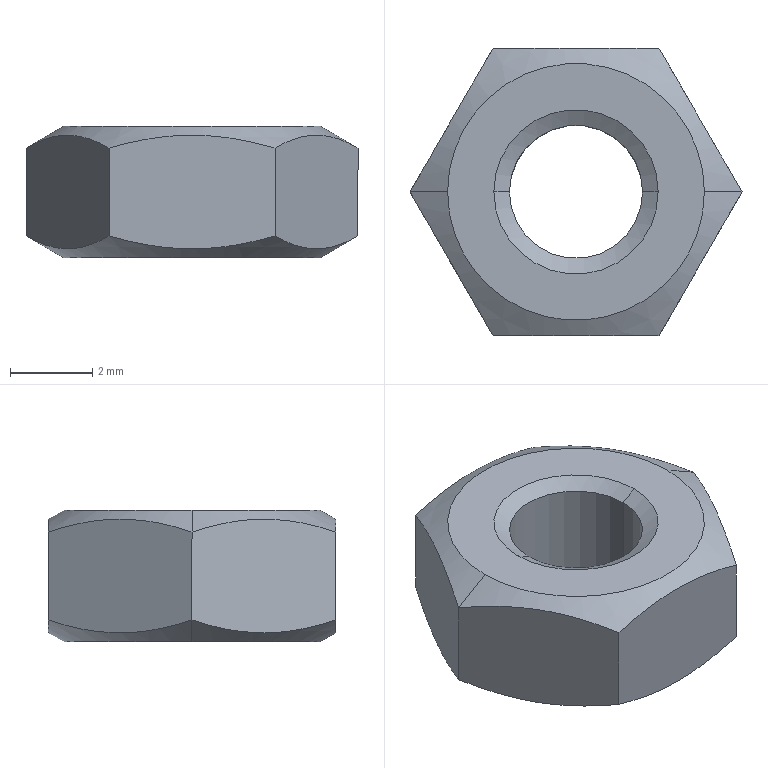Part | SolidWorks | features RevCut 2, Chamfer 1, Extrusion 1, LPattern 1 | 1 solid | 18 faces | box 8.083 x 7 x 3.2 mm | volume 104.299 mm3 | cone 8 | plane 8 | cylinder 2 | commonest cylinder face diameters 3.242 x2
STEP:
#1=CARTESIAN_POINT('',(-1.621,0.,-0.2188));
#2=VERTEX_POINT('',#1);
#3=CARTESIAN_POINT('',(1.621,0.,-0.2188));
#4=VERTEX_POINT('',#3);
#5=CARTESIAN_POINT('',(0.,0.,-0.2188));
#6=DIRECTION('',(0.,0.,1.));
#7=DIRECTION('',(-1.,0.,0.));
#8=AXIS2_PLACEMENT_3D('',#5,#6,#7);
#9=CIRCLE('',#8,1.621);
#10=EDGE_CURVE('',#2,#4,#9,.T.);
#11=ORIENTED_EDGE('',*,*,#10,.F.);
#12=CARTESIAN_POINT('',(-2.,0.,0.));
#13=VERTEX_POINT('',#12);
#14=CARTESIAN_POINT('',(-1.621,0.,-0.2188));
#15=DIRECTION('',(-0.866,0.,0.5));
#16=VECTOR('',#15,1000.);
#17=LINE('',#14,#16);
#18=EDGE_CURVE('',#2,#13,#17,.T.);
#19=ORIENTED_EDGE('',*,*,#18,.T.);
#20=CARTESIAN_POINT('',(2.,0.,0.));
#21=VERTEX_POINT('',#20);
#22=CARTESIAN_POINT('',(0.,0.,0.));
#23=DIRECTION('',(0.,0.,-1.));
#24=DIRECTION('',(-1.,0.,0.));
#25=AXIS2_PLACEMENT_3D('',#22,#23,#24);
#26=CIRCLE('',#25,2.);
#27=EDGE_CURVE('',#21,#13,#26,.T.);
#28=ORIENTED_EDGE('',*,*,#27,.F.);
#29=CARTESIAN_POINT('',(1.621,0.,-0.2188));
#30=DIRECTION('',(0.866,0.,0.5));
#31=VECTOR('',#30,1000.);
#32=LINE('',#29,#31);
#33=EDGE_CURVE('',#4,#21,#32,.T.);
#34=ORIENTED_EDGE('',*,*,#33,.F.);
#35=EDGE_LOOP('',(#11,#19,#28,#34));
#36=FACE_OUTER_BOUND('',#35,.T.);
#37=CARTESIAN_POINT('',(0.,0.,-0.2188));
#38=DIRECTION('',(0.,0.,1.));
#39=DIRECTION('',(1.,0.,0.));
#40=AXIS2_PLACEMENT_3D('',#37,#38,#39);
#41=CONICAL_SURFACE('',#40,1.621,1.047);
#42=ADVANCED_FACE('',(#36),#41,.F.);
#43=CARTESIAN_POINT('',(1.621,0.,-2.821));
#44=VERTEX_POINT('',#43);
#45=CARTESIAN_POINT('',(-1.621,0.,-2.821));
#46=VERTEX_POINT('',#45);
#47=CARTESIAN_POINT('',(0.,0.,-2.821));
#48=DIRECTION('',(0.,0.,-1.));
#49=DIRECTION('',(-1.,0.,0.));
#50=AXIS2_PLACEMENT_3D('',#47,#48,#49);
#51=CIRCLE('',#50,1.621);
#52=EDGE_CURVE('',#44,#46,#51,.T.);
#53=ORIENTED_EDGE('',*,*,#52,.F.);
#54=CARTESIAN_POINT('',(1.84,0.,-3.2));
#55=VERTEX_POINT('',#54);
#56=CARTESIAN_POINT('',(1.84,0.,-3.2));
#57=DIRECTION('',(0.5,0.,-0.866));
#58=VECTOR('',#57,1000.);
#59=LINE('',#56,#58);
#60=EDGE_CURVE('',#44,#55,#59,.T.);
#61=ORIENTED_EDGE('',*,*,#60,.T.);
#62=CARTESIAN_POINT('',(-1.84,0.,-3.2));
#63=VERTEX_POINT('',#62);
#64=CARTESIAN_POINT('',(0.,0.,-3.2));
#65=DIRECTION('',(0.,0.,1.));
#66=DIRECTION('',(-1.,0.,0.));
#67=AXIS2_PLACEMENT_3D('',#64,#65,#66);
#68=CIRCLE('',#67,1.84);
#69=EDGE_CURVE('',#63,#55,#68,.T.);
#70=ORIENTED_EDGE('',*,*,#69,.F.);
#71=CARTESIAN_POINT('',(-1.84,0.,-3.2));
#72=DIRECTION('',(-0.5,0.,-0.866));
#73=VECTOR('',#72,1000.);
#74=LINE('',#71,#73);
#75=EDGE_CURVE('',#46,#63,#74,.T.);
#76=ORIENTED_EDGE('',*,*,#75,.F.);
#77=EDGE_LOOP('',(#53,#61,#70,#76));
#78=FACE_OUTER_BOUND('',#77,.T.);
#79=CARTESIAN_POINT('',(0.,0.,-3.2));
#80=DIRECTION('',(0.,0.,-1.));
#81=DIRECTION('',(-1.,0.,0.));
#82=AXIS2_PLACEMENT_3D('',#79,#80,#81);
#83=CONICAL_SURFACE('',#82,1.84,0.5236);
#84=ADVANCED_FACE('',(#78),#83,.F.);
#85=CARTESIAN_POINT('',(-3.125,0.,0.));
#86=VERTEX_POINT('',#85);
#87=CARTESIAN_POINT('',(3.125,0.,0.));
#88=VERTEX_POINT('',#87);
#89=CARTESIAN_POINT('',(0.,0.,0.));
#90=DIRECTION('',(0.,0.,-1.));
#91=DIRECTION('',(-1.,0.,0.));
#92=AXIS2_PLACEMENT_3D('',#89,#90,#91);
#93=CIRCLE('',#92,3.125);
#94=EDGE_CURVE('',#86,#88,#93,.T.);
#95=ORIENTED_EDGE('',*,*,#94,.T.);
#96=CARTESIAN_POINT('',(4.041,0.,-0.5291));
#97=VERTEX_POINT('',#96);
#98=CARTESIAN_POINT('',(3.125,0.,0.));
#99=DIRECTION('',(0.866,0.,-0.5));
#100=VECTOR('',#99,1000.);
#101=LINE('',#98,#100);
#102=EDGE_CURVE('',#88,#97,#101,.T.);
#103=ORIENTED_EDGE('',*,*,#102,.T.);
#104=CARTESIAN_POINT('',(2.021,3.5,-0.5291));
#105=VERTEX_POINT('',#104);
#106=CARTESIAN_POINT('',(4.041,0.,-0.5291));
#107=CARTESIAN_POINT('',(3.712,0.5715,-0.3386));
#108=CARTESIAN_POINT('',(3.377,1.152,-0.2169));
#109=CARTESIAN_POINT('',(2.861,2.044,-0.2163));
#110=CARTESIAN_POINT('',(2.69,2.341,-0.2461));
#111=CARTESIAN_POINT('',(2.352,2.925,-0.3551));
#112=CARTESIAN_POINT('',(2.186,3.214,-0.4337));
#113=CARTESIAN_POINT('',(2.021,3.5,-0.5291));
#114=B_SPLINE_CURVE_WITH_KNOTS('',3,(#106,#107,#108,#109,#110,#111,#112,#113),.UNSPECIFIED.,.F.,.F.,(4,2,2,4),(0.000000238,0.002041,0.003061,0.004082),.UNSPECIFIED.);
#115=EDGE_CURVE('',#97,#105,#114,.T.);
#116=ORIENTED_EDGE('',*,*,#115,.T.);
#117=CARTESIAN_POINT('',(-2.021,3.5,-0.5291));
#118=VERTEX_POINT('',#117);
#119=CARTESIAN_POINT('',(2.021,3.5,-0.5291));
#120=CARTESIAN_POINT('',(1.694,3.5,-0.4348));
#121=CARTESIAN_POINT('',(1.363,3.5,-0.3563));
#122=CARTESIAN_POINT('',(0.6882,3.5,-0.2467));
#123=CARTESIAN_POINT('',(0.342,3.5,-0.2165));
#124=CARTESIAN_POINT('',(-0.3409,3.5,-0.2165));
#125=CARTESIAN_POINT('',(-0.6803,3.5,-0.2458));
#126=CARTESIAN_POINT('',(-1.355,3.5,-0.3546));
#127=CARTESIAN_POINT('',(-1.692,3.5,-0.4342));
#128=CARTESIAN_POINT('',(-2.021,3.5,-0.5291));
#129=B_SPLINE_CURVE_WITH_KNOTS('',3,(#119,#120,#121,#122,#123,#124,#125,#126,#127,#128),.UNSPECIFIED.,.F.,.F.,(4,2,2,2,4),(0.008992,0.01002,0.01104,0.01206,0.01309),.UNSPECIFIED.);
#130=EDGE_CURVE('',#105,#118,#129,.T.);
#131=ORIENTED_EDGE('',*,*,#130,.T.);
#132=CARTESIAN_POINT('',(-4.041,0.,-0.5291));
#133=VERTEX_POINT('',#132);
#134=CARTESIAN_POINT('',(-2.021,3.5,-0.5291));
#135=CARTESIAN_POINT('',(-2.351,2.929,-0.3386));
#136=CARTESIAN_POINT('',(-2.686,2.348,-0.2169));
#137=CARTESIAN_POINT('',(-3.201,1.456,-0.2163));
#138=CARTESIAN_POINT('',(-3.373,1.159,-0.2461));
#139=CARTESIAN_POINT('',(-3.71,0.5746,-0.3551));
#140=CARTESIAN_POINT('',(-3.876,0.2861,-0.4337));
#141=CARTESIAN_POINT('',(-4.041,0.,-0.5291));
#142=B_SPLINE_CURVE_WITH_KNOTS('',3,(#134,#135,#136,#137,#138,#139,#140,#141),.UNSPECIFIED.,.F.,.F.,(4,2,2,4),(0.000000238,0.002041,0.003061,0.004082),.UNSPECIFIED.);
#143=EDGE_CURVE('',#118,#133,#142,.T.);
#144=ORIENTED_EDGE('',*,*,#143,.T.);
#145=CARTESIAN_POINT('',(-3.125,0.,0.));
#146=DIRECTION('',(-0.866,0.,-0.5));
#147=VECTOR('',#146,1000.);
#148=LINE('',#145,#147);
#149=EDGE_CURVE('',#86,#133,#148,.T.);
#150=ORIENTED_EDGE('',*,*,#149,.F.);
#151=EDGE_LOOP('',(#95,#103,#116,#131,#144,#150));
#152=FACE_OUTER_BOUND('',#151,.T.);
#153=CARTESIAN_POINT('',(0.,0.,0.));
#154=DIRECTION('',(0.,0.,-1.));
#155=DIRECTION('',(-1.,0.,0.));
#156=AXIS2_PLACEMENT_3D('',#153,#154,#155);
#157=CONICAL_SURFACE('',#156,3.125,1.047);
#158=ADVANCED_FACE('',(#152),#157,.T.);
#159=CARTESIAN_POINT('',(-3.125,0.,-3.2));
#160=VERTEX_POINT('',#159);
#161=CARTESIAN_POINT('',(3.125,0.,-3.2));
#162=VERTEX_POINT('',#161);
#163=CARTESIAN_POINT('',(0.,0.,-3.2));
#164=DIRECTION('',(0.,0.,-1.));
#165=DIRECTION('',(-1.,0.,0.));
#166=AXIS2_PLACEMENT_3D('',#163,#164,#165);
#167=CIRCLE('',#166,3.125);
#168=EDGE_CURVE('',#160,#162,#167,.T.);
#169=ORIENTED_EDGE('',*,*,#168,.F.);
#170=CARTESIAN_POINT('',(-4.041,0.,-2.671));
#171=VERTEX_POINT('',#170);
#172=CARTESIAN_POINT('',(-4.041,0.,-2.671));
#173=DIRECTION('',(-0.866,0.,0.5));
#174=VECTOR('',#173,1000.);
#175=LINE('',#172,#174);
#176=EDGE_CURVE('',#160,#171,#175,.T.);
#177=ORIENTED_EDGE('',*,*,#176,.T.);
#178=CARTESIAN_POINT('',(-2.021,3.5,-2.671));
#179=VERTEX_POINT('',#178);
#180=CARTESIAN_POINT('',(-4.041,0.,-2.671));
#181=CARTESIAN_POINT('',(-3.712,0.5715,-2.861));
#182=CARTESIAN_POINT('',(-3.377,1.152,-2.983));
#183=CARTESIAN_POINT('',(-2.861,2.044,-2.984));
#184=CARTESIAN_POINT('',(-2.69,2.341,-2.954));
#185=CARTESIAN_POINT('',(-2.352,2.925,-2.845));
#186=CARTESIAN_POINT('',(-2.186,3.214,-2.766));
#187=CARTESIAN_POINT('',(-2.021,3.5,-2.671));
#188=B_SPLINE_CURVE_WITH_KNOTS('',3,(#180,#181,#182,#183,#184,#185,#186,#187),.UNSPECIFIED.,.F.,.F.,(4,2,2,4),(0.000000238,0.002041,0.003061,0.004082),.UNSPECIFIED.);
#189=EDGE_CURVE('',#171,#179,#188,.T.);
#190=ORIENTED_EDGE('',*,*,#189,.T.);
#191=CARTESIAN_POINT('',(2.021,3.5,-2.671));
#192=VERTEX_POINT('',#191);
#193=CARTESIAN_POINT('',(-2.021,3.5,-2.671));
#194=CARTESIAN_POINT('',(-1.692,3.5,-2.766));
#195=CARTESIAN_POINT('',(-1.355,3.5,-2.845));
#196=CARTESIAN_POINT('',(-0.6803,3.5,-2.954));
#197=CARTESIAN_POINT('',(-0.3409,3.5,-2.984));
#198=CARTESIAN_POINT('',(0.342,3.5,-2.983));
#199=CARTESIAN_POINT('',(0.6882,3.5,-2.953));
#200=CARTESIAN_POINT('',(1.363,3.5,-2.844));
#201=CARTESIAN_POINT('',(1.694,3.5,-2.765));
#202=CARTESIAN_POINT('',(2.021,3.5,-2.671));
#203=B_SPLINE_CURVE_WITH_KNOTS('',3,(#193,#194,#195,#196,#197,#198,#199,#200,#201,#202),.UNSPECIFIED.,.F.,.F.,(4,2,2,2,4),(0.003572,0.004594,0.005616,0.006639,0.007661),.UNSPECIFIED.);
#204=EDGE_CURVE('',#179,#192,#203,.T.);
#205=ORIENTED_EDGE('',*,*,#204,.T.);
#206=CARTESIAN_POINT('',(4.041,0.,-2.671));
#207=VERTEX_POINT('',#206);
#208=CARTESIAN_POINT('',(2.021,3.5,-2.671));
#209=CARTESIAN_POINT('',(2.351,2.929,-2.861));
#210=CARTESIAN_POINT('',(2.686,2.348,-2.983));
#211=CARTESIAN_POINT('',(3.201,1.456,-2.984));
#212=CARTESIAN_POINT('',(3.373,1.159,-2.954));
#213=CARTESIAN_POINT('',(3.71,0.5746,-2.845));
#214=CARTESIAN_POINT('',(3.876,0.2861,-2.766));
#215=CARTESIAN_POINT('',(4.041,0.,-2.671));
#216=B_SPLINE_CURVE_WITH_KNOTS('',3,(#208,#209,#210,#211,#212,#213,#214,#215),.UNSPECIFIED.,.F.,.F.,(4,2,2,4),(0.000000238,0.002041,0.003061,0.004082),.UNSPECIFIED.);
#217=EDGE_CURVE('',#192,#207,#216,.T.);
#218=ORIENTED_EDGE('',*,*,#217,.T.);
#219=CARTESIAN_POINT('',(4.041,0.,-2.671));
#220=DIRECTION('',(0.866,0.,0.5));
#221=VECTOR('',#220,1000.);
#222=LINE('',#219,#221);
#223=EDGE_CURVE('',#162,#207,#222,.T.);
#224=ORIENTED_EDGE('',*,*,#223,.F.);
#225=EDGE_LOOP('',(#169,#177,#190,#205,#218,#224));
#226=FACE_OUTER_BOUND('',#225,.T.);
#227=CARTESIAN_POINT('',(0.,0.,-2.671));
#228=DIRECTION('',(0.,0.,1.));
#229=DIRECTION('',(1.,0.,0.));
#230=AXIS2_PLACEMENT_3D('',#227,#228,#229);
#231=CONICAL_SURFACE('',#230,4.041,1.047);
#232=ADVANCED_FACE('',(#226),#231,.T.);
#233=ORIENTED_EDGE('',*,*,#52,.T.);
#234=CARTESIAN_POINT('',(-1.621,0.,-3.2));
#235=DIRECTION('',(0.,0.,1.));
#236=VECTOR('',#235,1000.);
#237=LINE('',#234,#236);
#238=EDGE_CURVE('',#46,#2,#237,.T.);
#239=ORIENTED_EDGE('',*,*,#238,.T.);
#240=ORIENTED_EDGE('',*,*,#10,.T.);
#241=CARTESIAN_POINT('',(1.621,0.,-3.2));
#242=DIRECTION('',(0.,0.,1.));
#243=VECTOR('',#242,1000.);
#244=LINE('',#241,#243);
#245=EDGE_CURVE('',#44,#4,#244,.T.);
#246=ORIENTED_EDGE('',*,*,#245,.F.);
#247=EDGE_LOOP('',(#233,#239,#240,#246));
#248=FACE_OUTER_BOUND('',#247,.T.);
#249=CARTESIAN_POINT('',(0.,0.,-3.2));
#250=DIRECTION('',(0.,0.,1.));
#251=DIRECTION('',(1.,0.,0.));
#252=AXIS2_PLACEMENT_3D('',#249,#250,#251);
#253=CYLINDRICAL_SURFACE('',#252,1.621);
#254=ADVANCED_FACE('',(#248),#253,.F.);
#255=CARTESIAN_POINT('',(2.021,-3.5,-0.5291));
#256=VERTEX_POINT('',#255);
#257=CARTESIAN_POINT('',(2.021,-3.5,-0.5291));
#258=CARTESIAN_POINT('',(2.351,-2.929,-0.3386));
#259=CARTESIAN_POINT('',(2.686,-2.348,-0.2169));
#260=CARTESIAN_POINT('',(3.201,-1.456,-0.2163));
#261=CARTESIAN_POINT('',(3.373,-1.159,-0.2461));
#262=CARTESIAN_POINT('',(3.71,-0.5746,-0.3551));
#263=CARTESIAN_POINT('',(3.876,-0.2861,-0.4337));
#264=CARTESIAN_POINT('',(4.041,0.,-0.5291));
#265=B_SPLINE_CURVE_WITH_KNOTS('',3,(#257,#258,#259,#260,#261,#262,#263,#264),.UNSPECIFIED.,.F.,.F.,(4,2,2,4),(0.000000238,0.002041,0.003061,0.004082),.UNSPECIFIED.);
#266=EDGE_CURVE('',#256,#97,#265,.T.);
#267=ORIENTED_EDGE('',*,*,#266,.F.);
#268=CARTESIAN_POINT('',(2.021,-3.5,-2.671));
#269=VERTEX_POINT('',#268);
#270=CARTESIAN_POINT('',(2.021,-3.5,-3.2));
#271=DIRECTION('',(0.,0.,1.));
#272=VECTOR('',#271,1000.);
#273=LINE('',#270,#272);
#274=EDGE_CURVE('',#269,#256,#273,.T.);
#275=ORIENTED_EDGE('',*,*,#274,.F.);
#276=CARTESIAN_POINT('',(4.041,0.,-2.671));
#277=CARTESIAN_POINT('',(3.712,-0.5715,-2.861));
#278=CARTESIAN_POINT('',(3.377,-1.152,-2.983));
#279=CARTESIAN_POINT('',(2.861,-2.044,-2.984));
#280=CARTESIAN_POINT('',(2.69,-2.341,-2.954));
#281=CARTESIAN_POINT('',(2.352,-2.925,-2.845));
#282=CARTESIAN_POINT('',(2.186,-3.214,-2.766));
#283=CARTESIAN_POINT('',(2.021,-3.5,-2.671));
#284=B_SPLINE_CURVE_WITH_KNOTS('',3,(#276,#277,#278,#279,#280,#281,#282,#283),.UNSPECIFIED.,.F.,.F.,(4,2,2,4),(0.000000238,0.002041,0.003061,0.004082),.UNSPECIFIED.);
#285=EDGE_CURVE('',#207,#269,#284,.T.);
#286=ORIENTED_EDGE('',*,*,#285,.F.);
#287=CARTESIAN_POINT('',(4.041,0.,-3.2));
#288=DIRECTION('',(0.,0.,1.));
#289=VECTOR('',#288,1000.);
#290=LINE('',#287,#289);
#291=EDGE_CURVE('',#207,#97,#290,.T.);
#292=ORIENTED_EDGE('',*,*,#291,.T.);
#293=EDGE_LOOP('',(#267,#275,#286,#292));
#294=FACE_OUTER_BOUND('',#293,.T.);
#295=CARTESIAN_POINT('',(2.021,-3.5,-3.2));
#296=DIRECTION('',(0.866,-0.5,0.));
#297=DIRECTION('',(0.5,0.866,0.));
#298=AXIS2_PLACEMENT_3D('',#295,#296,#297);
#299=PLANE('',#298);
#300=ADVANCED_FACE('',(#294),#299,.T.);
#301=CARTESIAN_POINT('',(-2.021,-3.5,-0.5291));
#302=VERTEX_POINT('',#301);
#303=CARTESIAN_POINT('',(-2.021,-3.5,-0.5291));
#304=CARTESIAN_POINT('',(-1.692,-3.5,-0.4342));
#305=CARTESIAN_POINT('',(-1.355,-3.5,-0.3546));
#306=CARTESIAN_POINT('',(-0.6803,-3.5,-0.2458));
#307=CARTESIAN_POINT('',(-0.3409,-3.5,-0.2165));
#308=CARTESIAN_POINT('',(0.342,-3.5,-0.2165));
#309=CARTESIAN_POINT('',(0.6882,-3.5,-0.2467));
#310=CARTESIAN_POINT('',(1.363,-3.5,-0.3563));
#311=CARTESIAN_POINT('',(1.694,-3.5,-0.4348));
#312=CARTESIAN_POINT('',(2.021,-3.5,-0.5291));
#313=B_SPLINE_CURVE_WITH_KNOTS('',3,(#303,#304,#305,#306,#307,#308,#309,#310,#311,#312),.UNSPECIFIED.,.F.,.F.,(4,2,2,2,4),(0.003572,0.004594,0.005616,0.006639,0.007661),.UNSPECIFIED.);
#314=EDGE_CURVE('',#302,#256,#313,.T.);
#315=ORIENTED_EDGE('',*,*,#314,.F.);
#316=CARTESIAN_POINT('',(-2.021,-3.5,-2.671));
#317=VERTEX_POINT('',#316);
#318=CARTESIAN_POINT('',(-2.021,-3.5,-3.2));
#319=DIRECTION('',(0.,0.,1.));
#320=VECTOR('',#319,1000.);
#321=LINE('',#318,#320);
#322=EDGE_CURVE('',#317,#302,#321,.T.);
#323=ORIENTED_EDGE('',*,*,#322,.F.);
#324=CARTESIAN_POINT('',(2.021,-3.5,-2.671));
#325=CARTESIAN_POINT('',(1.694,-3.5,-2.765));
#326=CARTESIAN_POINT('',(1.363,-3.5,-2.844));
#327=CARTESIAN_POINT('',(0.6882,-3.5,-2.953));
#328=CARTESIAN_POINT('',(0.342,-3.5,-2.983));
#329=CARTESIAN_POINT('',(-0.3409,-3.5,-2.984));
#330=CARTESIAN_POINT('',(-0.6803,-3.5,-2.954));
#331=CARTESIAN_POINT('',(-1.355,-3.5,-2.845));
#332=CARTESIAN_POINT('',(-1.692,-3.5,-2.766));
#333=CARTESIAN_POINT('',(-2.021,-3.5,-2.671));
#334=B_SPLINE_CURVE_WITH_KNOTS('',3,(#324,#325,#326,#327,#328,#329,#330,#331,#332,#333),.UNSPECIFIED.,.F.,.F.,(4,2,2,2,4),(0.008992,0.01002,0.01104,0.01206,0.01309),.UNSPECIFIED.);
#335=EDGE_CURVE('',#269,#317,#334,.T.);
#336=ORIENTED_EDGE('',*,*,#335,.F.);
#337=ORIENTED_EDGE('',*,*,#274,.T.);
#338=EDGE_LOOP('',(#315,#323,#336,#337));
#339=FACE_OUTER_BOUND('',#338,.T.);
#340=CARTESIAN_POINT('',(-2.021,-3.5,-3.2));
#341=DIRECTION('',(0.,-1.,0.));
#342=DIRECTION('',(1.,0.,0.));
#343=AXIS2_PLACEMENT_3D('',#340,#341,#342);
#344=PLANE('',#343);
#345=ADVANCED_FACE('',(#339),#344,.T.);
#346=CARTESIAN_POINT('',(-4.041,0.,-0.5291));
#347=CARTESIAN_POINT('',(-3.712,-0.5715,-0.3386));
#348=CARTESIAN_POINT('',(-3.377,-1.152,-0.2169));
#349=CARTESIAN_POINT('',(-2.861,-2.044,-0.2163));
#350=CARTESIAN_POINT('',(-2.69,-2.341,-0.2461));
#351=CARTESIAN_POINT('',(-2.352,-2.925,-0.3551));
#352=CARTESIAN_POINT('',(-2.186,-3.214,-0.4337));
#353=CARTESIAN_POINT('',(-2.021,-3.5,-0.5291));
#354=B_SPLINE_CURVE_WITH_KNOTS('',3,(#346,#347,#348,#349,#350,#351,#352,#353),.UNSPECIFIED.,.F.,.F.,(4,2,2,4),(0.000000238,0.002041,0.003061,0.004082),.UNSPECIFIED.);
#355=EDGE_CURVE('',#133,#302,#354,.T.);
#356=ORIENTED_EDGE('',*,*,#355,.F.);
#357=CARTESIAN_POINT('',(-4.041,0.,-3.2));
#358=DIRECTION('',(0.,0.,1.));
#359=VECTOR('',#358,1000.);
#360=LINE('',#357,#359);
#361=EDGE_CURVE('',#171,#133,#360,.T.);
#362=ORIENTED_EDGE('',*,*,#361,.F.);
#363=CARTESIAN_POINT('',(-2.021,-3.5,-2.671));
#364=CARTESIAN_POINT('',(-2.351,-2.929,-2.861));
#365=CARTESIAN_POINT('',(-2.686,-2.348,-2.983));
#366=CARTESIAN_POINT('',(-3.201,-1.456,-2.984));
#367=CARTESIAN_POINT('',(-3.373,-1.159,-2.954));
#368=CARTESIAN_POINT('',(-3.71,-0.5746,-2.845));
#369=CARTESIAN_POINT('',(-3.876,-0.2861,-2.766));
#370=CARTESIAN_POINT('',(-4.041,0.,-2.671));
#371=B_SPLINE_CURVE_WITH_KNOTS('',3,(#363,#364,#365,#366,#367,#368,#369,#370),.UNSPECIFIED.,.F.,.F.,(4,2,2,4),(0.000000238,0.002041,0.003061,0.004082),.UNSPECIFIED.);
#372=EDGE_CURVE('',#317,#171,#371,.T.);
#373=ORIENTED_EDGE('',*,*,#372,.F.);
#374=ORIENTED_EDGE('',*,*,#322,.T.);
#375=EDGE_LOOP('',(#356,#362,#373,#374));
#376=FACE_OUTER_BOUND('',#375,.T.);
#377=CARTESIAN_POINT('',(-4.041,0.,-3.2));
#378=DIRECTION('',(-0.866,-0.5,0.));
#379=DIRECTION('',(0.5,-0.866,0.));
#380=AXIS2_PLACEMENT_3D('',#377,#378,#379);
#381=PLANE('',#380);
#382=ADVANCED_FACE('',(#376),#381,.T.);
#383=ORIENTED_EDGE('',*,*,#143,.F.);
#384=CARTESIAN_POINT('',(-2.021,3.5,-3.2));
#385=DIRECTION('',(0.,0.,1.));
#386=VECTOR('',#385,1000.);
#387=LINE('',#384,#386);
#388=EDGE_CURVE('',#179,#118,#387,.T.);
#389=ORIENTED_EDGE('',*,*,#388,.F.);
#390=ORIENTED_EDGE('',*,*,#189,.F.);
#391=ORIENTED_EDGE('',*,*,#361,.T.);
#392=EDGE_LOOP('',(#383,#389,#390,#391));
#393=FACE_OUTER_BOUND('',#392,.T.);
#394=CARTESIAN_POINT('',(-2.021,3.5,-3.2));
#395=DIRECTION('',(-0.866,0.5,0.));
#396=DIRECTION('',(-0.5,-0.866,0.));
#397=AXIS2_PLACEMENT_3D('',#394,#395,#396);
#398=PLANE('',#397);
#399=ADVANCED_FACE('',(#393),#398,.T.);
#400=ORIENTED_EDGE('',*,*,#130,.F.);
#401=CARTESIAN_POINT('',(2.021,3.5,-3.2));
#402=DIRECTION('',(0.,0.,1.));
#403=VECTOR('',#402,1000.);
#404=LINE('',#401,#403);
#405=EDGE_CURVE('',#192,#105,#404,.T.);
#406=ORIENTED_EDGE('',*,*,#405,.F.);
#407=ORIENTED_EDGE('',*,*,#204,.F.);
#408=ORIENTED_EDGE('',*,*,#388,.T.);
#409=EDGE_LOOP('',(#400,#406,#407,#408));
#410=FACE_OUTER_BOUND('',#409,.T.);
#411=CARTESIAN_POINT('',(2.021,3.5,-3.2));
#412=DIRECTION('',(0.,1.,0.));
#413=DIRECTION('',(0.,0.,1.));
#414=AXIS2_PLACEMENT_3D('',#411,#412,#413);
#415=PLANE('',#414);
#416=ADVANCED_FACE('',(#410),#415,.T.);
#417=ORIENTED_EDGE('',*,*,#115,.F.);
#418=ORIENTED_EDGE('',*,*,#291,.F.);
#419=ORIENTED_EDGE('',*,*,#217,.F.);
#420=ORIENTED_EDGE('',*,*,#405,.T.);
#421=EDGE_LOOP('',(#417,#418,#419,#420));
#422=FACE_OUTER_BOUND('',#421,.T.);
#423=CARTESIAN_POINT('',(4.041,0.,-3.2));
#424=DIRECTION('',(0.866,0.5,0.));
#425=DIRECTION('',(-0.5,0.866,0.));
#426=AXIS2_PLACEMENT_3D('',#423,#424,#425);
#427=PLANE('',#426);
#428=ADVANCED_FACE('',(#422),#427,.T.);
#429=ORIENTED_EDGE('',*,*,#69,.T.);
#430=CARTESIAN_POINT('',(0.,0.,-3.2));
#431=DIRECTION('',(0.,0.,1.));
#432=DIRECTION('',(-1.,0.,0.));
#433=AXIS2_PLACEMENT_3D('',#430,#431,#432);
#434=CIRCLE('',#433,1.84);
#435=EDGE_CURVE('',#55,#63,#434,.T.);
#436=ORIENTED_EDGE('',*,*,#435,.T.);
#437=EDGE_LOOP('',(#429,#436));
#438=FACE_BOUND('',#437,.T.);
#439=CARTESIAN_POINT('',(0.,0.,-3.2));
#440=DIRECTION('',(0.,0.,-1.));
#441=DIRECTION('',(-1.,0.,0.));
#442=AXIS2_PLACEMENT_3D('',#439,#440,#441);
#443=CIRCLE('',#442,3.125);
#444=EDGE_CURVE('',#162,#160,#443,.T.);
#445=ORIENTED_EDGE('',*,*,#444,.T.);
#446=ORIENTED_EDGE('',*,*,#168,.T.);
#447=EDGE_LOOP('',(#445,#446));
#448=FACE_OUTER_BOUND('',#447,.T.);
#449=CARTESIAN_POINT('',(2.021,-3.5,-3.2));
#450=DIRECTION('',(0.,0.,-1.));
#451=DIRECTION('',(-1.,0.,0.));
#452=AXIS2_PLACEMENT_3D('',#449,#450,#451);
#453=PLANE('',#452);
#454=ADVANCED_FACE('',(#438,#448),#453,.T.);
#455=ORIENTED_EDGE('',*,*,#27,.T.);
#456=CARTESIAN_POINT('',(0.,0.,0.));
#457=DIRECTION('',(0.,0.,-1.));
#458=DIRECTION('',(-1.,0.,0.));
#459=AXIS2_PLACEMENT_3D('',#456,#457,#458);
#460=CIRCLE('',#459,2.);
#461=EDGE_CURVE('',#13,#21,#460,.T.);
#462=ORIENTED_EDGE('',*,*,#461,.T.);
#463=EDGE_LOOP('',(#455,#462));
#464=FACE_BOUND('',#463,.T.);
#465=ORIENTED_EDGE('',*,*,#94,.F.);
#466=CARTESIAN_POINT('',(0.,0.,0.));
#467=DIRECTION('',(0.,0.,-1.));
#468=DIRECTION('',(-1.,0.,0.));
#469=AXIS2_PLACEMENT_3D('',#466,#467,#468);
#470=CIRCLE('',#469,3.125);
#471=EDGE_CURVE('',#88,#86,#470,.T.);
#472=ORIENTED_EDGE('',*,*,#471,.F.);
#473=EDGE_LOOP('',(#465,#472));
#474=FACE_OUTER_BOUND('',#473,.T.);
#475=CARTESIAN_POINT('',(2.021,-3.5,0.));
#476=DIRECTION('',(0.,0.,-1.));
#477=DIRECTION('',(-1.,0.,0.));
#478=AXIS2_PLACEMENT_3D('',#475,#476,#477);
#479=PLANE('',#478);
#480=ADVANCED_FACE('',(#464,#474),#479,.F.);
#481=ORIENTED_EDGE('',*,*,#238,.F.);
#482=CARTESIAN_POINT('',(0.,0.,-2.821));
#483=DIRECTION('',(0.,0.,-1.));
#484=DIRECTION('',(-1.,0.,0.));
#485=AXIS2_PLACEMENT_3D('',#482,#483,#484);
#486=CIRCLE('',#485,1.621);
#487=EDGE_CURVE('',#46,#44,#486,.T.);
#488=ORIENTED_EDGE('',*,*,#487,.T.);
#489=ORIENTED_EDGE('',*,*,#245,.T.);
#490=CARTESIAN_POINT('',(0.,0.,-0.2188));
#491=DIRECTION('',(0.,0.,1.));
#492=DIRECTION('',(-1.,0.,0.));
#493=AXIS2_PLACEMENT_3D('',#490,#491,#492);
#494=CIRCLE('',#493,1.621);
#495=EDGE_CURVE('',#4,#2,#494,.T.);
#496=ORIENTED_EDGE('',*,*,#495,.T.);
#497=EDGE_LOOP('',(#481,#488,#489,#496));
#498=FACE_OUTER_BOUND('',#497,.T.);
#499=CARTESIAN_POINT('',(0.,0.,-3.2));
#500=DIRECTION('',(0.,0.,1.));
#501=DIRECTION('',(1.,0.,0.));
#502=AXIS2_PLACEMENT_3D('',#499,#500,#501);
#503=CYLINDRICAL_SURFACE('',#502,1.621);
#504=ADVANCED_FACE('',(#498),#503,.F.);
#505=ORIENTED_EDGE('',*,*,#176,.F.);
#506=ORIENTED_EDGE('',*,*,#444,.F.);
#507=ORIENTED_EDGE('',*,*,#223,.T.);
#508=ORIENTED_EDGE('',*,*,#285,.T.);
#509=ORIENTED_EDGE('',*,*,#335,.T.);
#510=ORIENTED_EDGE('',*,*,#372,.T.);
#511=EDGE_LOOP('',(#505,#506,#507,#508,#509,#510));
#512=FACE_OUTER_BOUND('',#511,.T.);
#513=CARTESIAN_POINT('',(0.,0.,-2.671));
#514=DIRECTION('',(0.,0.,1.));
#515=DIRECTION('',(1.,0.,0.));
#516=AXIS2_PLACEMENT_3D('',#513,#514,#515);
#517=CONICAL_SURFACE('',#516,4.041,1.047);
#518=ADVANCED_FACE('',(#512),#517,.T.);
#519=ORIENTED_EDGE('',*,*,#102,.F.);
#520=ORIENTED_EDGE('',*,*,#471,.T.);
#521=ORIENTED_EDGE('',*,*,#149,.T.);
#522=ORIENTED_EDGE('',*,*,#355,.T.);
#523=ORIENTED_EDGE('',*,*,#314,.T.);
#524=ORIENTED_EDGE('',*,*,#266,.T.);
#525=EDGE_LOOP('',(#519,#520,#521,#522,#523,#524));
#526=FACE_OUTER_BOUND('',#525,.T.);
#527=CARTESIAN_POINT('',(0.,0.,0.));
#528=DIRECTION('',(0.,0.,-1.));
#529=DIRECTION('',(-1.,0.,0.));
#530=AXIS2_PLACEMENT_3D('',#527,#528,#529);
#531=CONICAL_SURFACE('',#530,3.125,1.047);
#532=ADVANCED_FACE('',(#526),#531,.T.);
#533=ORIENTED_EDGE('',*,*,#60,.F.);
#534=ORIENTED_EDGE('',*,*,#487,.F.);
#535=ORIENTED_EDGE('',*,*,#75,.T.);
#536=ORIENTED_EDGE('',*,*,#435,.F.);
#537=EDGE_LOOP('',(#533,#534,#535,#536));
#538=FACE_OUTER_BOUND('',#537,.T.);
#539=CARTESIAN_POINT('',(0.,0.,-3.2));
#540=DIRECTION('',(0.,0.,-1.));
#541=DIRECTION('',(-1.,0.,0.));
#542=AXIS2_PLACEMENT_3D('',#539,#540,#541);
#543=CONICAL_SURFACE('',#542,1.84,0.5236);
#544=ADVANCED_FACE('',(#538),#543,.F.);
#545=ORIENTED_EDGE('',*,*,#18,.F.);
#546=ORIENTED_EDGE('',*,*,#495,.F.);
#547=ORIENTED_EDGE('',*,*,#33,.T.);
#548=ORIENTED_EDGE('',*,*,#461,.F.);
#549=EDGE_LOOP('',(#545,#546,#547,#548));
#550=FACE_OUTER_BOUND('',#549,.T.);
#551=CARTESIAN_POINT('',(0.,0.,-0.2188));
#552=DIRECTION('',(0.,0.,1.));
#553=DIRECTION('',(1.,0.,0.));
#554=AXIS2_PLACEMENT_3D('',#551,#552,#553);
#555=CONICAL_SURFACE('',#554,1.621,1.047);
#556=ADVANCED_FACE('',(#550),#555,.F.);
#557=CLOSED_SHELL('',(#42,#84,#158,#232,#254,#300,#345,#382,#399,#416,#428,#454,#480,#504,#518,#532,#544,#556));
#558=MANIFOLD_SOLID_BREP('',#557);
#559=CARTESIAN_POINT('',(0.,0.,0.));
#560=DIRECTION('',(0.,0.,1.));
#561=DIRECTION('',(1.,0.,0.));
#562=AXIS2_PLACEMENT_3D('',#559,#560,#561);
#563=(LENGTH_UNIT()NAMED_UNIT(*)SI_UNIT(.MILLI.,.METRE.));
#564=UNCERTAINTY_MEASURE_WITH_UNIT(LENGTH_MEASURE(0.00001),#563,'','');
#565=(NAMED_UNIT(*)PLANE_ANGLE_UNIT()SI_UNIT($,.RADIAN.));
#566=(NAMED_UNIT(*)SI_UNIT($,.STERADIAN.)SOLID_ANGLE_UNIT());
#567=(GEOMETRIC_REPRESENTATION_CONTEXT(3)GLOBAL_UNCERTAINTY_ASSIGNED_CONTEXT((#564))GLOBAL_UNIT_ASSIGNED_CONTEXT((#563,#565,#566))REPRESENTATION_CONTEXT('',''));
#568=ADVANCED_BREP_SHAPE_REPRESENTATION('',(#558,#562),#567);